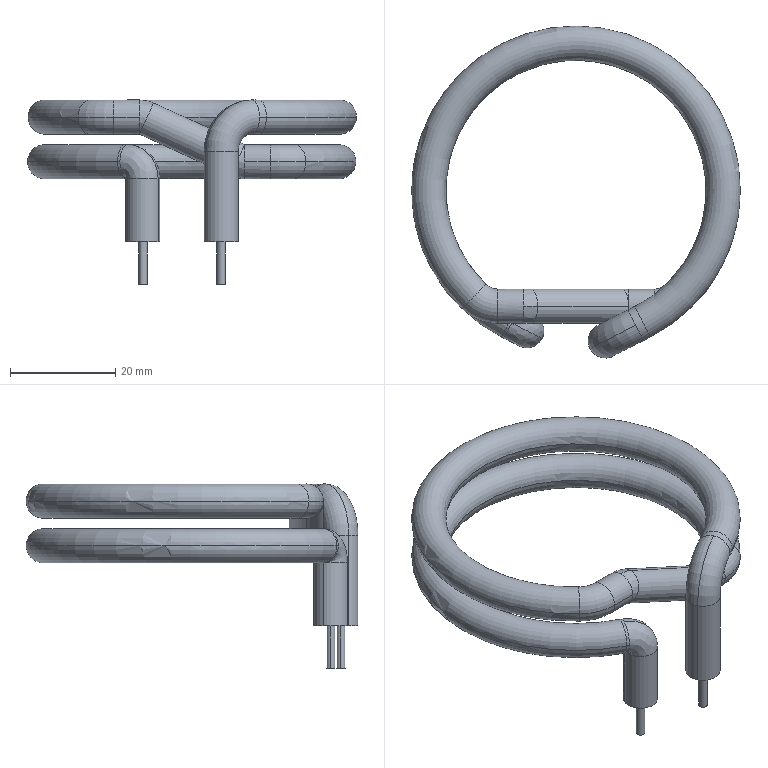Part | STEP file | JIAREQI_2_1_1_1 | 1 solid | 38 faces | box 62.5 x 63.088 x 35 mm | volume 12336 mm3 | cylinder 18 | torus 10 | spline 6 | plane 4 | commonest cylinder face diameters 6.5 x14 1.6 x4
STEP:
#1=CARTESIAN_POINT('',(0.,0.,0.));
#2=DIRECTION('',(0.,0.,1.));
#3=DIRECTION('',(1.,0.,0.));
#4=AXIS2_PLACEMENT_3D('',#1,#2,#3);
#5=CARTESIAN_POINT('',(11.339,-25.645,3.25));
#6=VERTEX_POINT('',#5);
#7=CARTESIAN_POINT('',(12.811,-28.543,0.));
#8=VERTEX_POINT('',#7);
#9=CARTESIAN_POINT('',(11.339,-25.645,0.));
#10=DIRECTION('',(0.8916,0.4527,0.));
#11=DIRECTION('',(0.,0.,1.));
#12=AXIS2_PLACEMENT_3D('',#9,#10,#11);
#13=CIRCLE('',#12,3.25);
#14=EDGE_CURVE('',#6,#8,#13,.T.);
#15=ORIENTED_EDGE('',*,*,#14,.F.);
#16=CARTESIAN_POINT('',(9.868,-22.747,0.));
#17=VERTEX_POINT('',#16);
#18=CARTESIAN_POINT('',(11.339,-25.645,0.));
#19=DIRECTION('',(0.8916,0.4527,0.));
#20=DIRECTION('',(-0.4527,0.8916,0.));
#21=AXIS2_PLACEMENT_3D('',#18,#19,#20);
#22=CIRCLE('',#21,3.25);
#23=EDGE_CURVE('',#17,#6,#22,.T.);
#24=ORIENTED_EDGE('',*,*,#23,.F.);
#25=CARTESIAN_POINT('',(11.206,-22.068,0.));
#26=VERTEX_POINT('',#25);
#27=CARTESIAN_POINT('',(9.868,-22.747,0.));
#28=DIRECTION('',(0.8916,0.4527,0.));
#29=VECTOR('',#28,1.5);
#30=LINE('',#27,#29);
#31=EDGE_CURVE('',#17,#26,#30,.T.);
#32=ORIENTED_EDGE('',*,*,#31,.T.);
#33=CARTESIAN_POINT('',(14.148,-27.864,0.));
#34=VERTEX_POINT('',#33);
#35=CARTESIAN_POINT('',(12.677,-24.966,0.));
#36=DIRECTION('',(-0.8916,-0.4527,0.));
#37=DIRECTION('',(0.4527,-0.8916,0.));
#38=AXIS2_PLACEMENT_3D('',#35,#36,#37);
#39=CIRCLE('',#38,3.25);
#40=EDGE_CURVE('',#34,#26,#39,.T.);
#41=ORIENTED_EDGE('',*,*,#40,.F.);
#42=CARTESIAN_POINT('',(12.811,-28.543,0.));
#43=DIRECTION('',(0.8916,0.4527,0.));
#44=VECTOR('',#43,1.5);
#45=LINE('',#42,#44);
#46=EDGE_CURVE('',#8,#34,#45,.T.);
#47=ORIENTED_EDGE('',*,*,#46,.F.);
#48=EDGE_LOOP('',(#15,#24,#32,#41,#47));
#49=FACE_OUTER_BOUND('',#48,.F.);
#50=CARTESIAN_POINT('',(11.339,-25.645,0.));
#51=DIRECTION('',(0.8916,0.4527,0.));
#52=DIRECTION('',(-0.4527,0.8916,0.));
#53=AXIS2_PLACEMENT_3D('',#50,#51,#52);
#54=CYLINDRICAL_SURFACE('',#53,3.25);
#55=ADVANCED_FACE('',(#49),#54,.T.);
#56=ORIENTED_EDGE('',*,*,#14,.T.);
#57=CARTESIAN_POINT('',(11.339,-25.645,-3.25));
#58=VERTEX_POINT('',#57);
#59=CARTESIAN_POINT('',(11.339,-25.645,0.));
#60=DIRECTION('',(0.8916,0.4527,0.));
#61=DIRECTION('',(0.4527,-0.8916,0.));
#62=AXIS2_PLACEMENT_3D('',#59,#60,#61);
#63=CIRCLE('',#62,3.25);
#64=EDGE_CURVE('',#8,#58,#63,.T.);
#65=ORIENTED_EDGE('',*,*,#64,.T.);
#66=CARTESIAN_POINT('',(8.442,-27.116,-6.5));
#67=VERTEX_POINT('',#66);
#68=CARTESIAN_POINT('',(11.339,-25.645,-6.5));
#69=DIRECTION('',(0.4527,-0.8916,0.));
#70=DIRECTION('',(0.,0.,1.));
#71=AXIS2_PLACEMENT_3D('',#68,#69,#70);
#72=CIRCLE('',#71,3.25);
#73=EDGE_CURVE('',#58,#67,#72,.T.);
#74=ORIENTED_EDGE('',*,*,#73,.T.);
#75=CARTESIAN_POINT('',(2.646,-30.059,-6.5));
#76=VERTEX_POINT('',#75);
#77=CARTESIAN_POINT('',(5.544,-28.588,-6.5));
#78=DIRECTION('',(0.,0.,-1.));
#79=DIRECTION('',(0.8916,0.4527,0.));
#80=AXIS2_PLACEMENT_3D('',#77,#78,#79);
#81=CIRCLE('',#80,3.25);
#82=EDGE_CURVE('',#67,#76,#81,.T.);
#83=ORIENTED_EDGE('',*,*,#82,.T.);
#84=CARTESIAN_POINT('',(11.339,-25.645,-6.5));
#85=DIRECTION('',(0.4527,-0.8916,0.));
#86=DIRECTION('',(0.,0.,1.));
#87=AXIS2_PLACEMENT_3D('',#84,#85,#86);
#88=CIRCLE('',#87,9.75);
#89=EDGE_CURVE('',#6,#76,#88,.T.);
#90=ORIENTED_EDGE('',*,*,#89,.F.);
#91=EDGE_LOOP('',(#56,#65,#74,#83,#90));
#92=FACE_OUTER_BOUND('',#91,.F.);
#93=CARTESIAN_POINT('',(11.339,-25.645,-6.5));
#94=DIRECTION('',(0.4527,-0.8916,0.));
#95=DIRECTION('',(0.,0.,-1.));
#96=AXIS2_PLACEMENT_3D('',#93,#94,#95);
#97=TOROIDAL_SURFACE('',#96,6.5,3.25);
#98=ADVANCED_FACE('',(#92),#97,.T.);
#99=ORIENTED_EDGE('',*,*,#64,.F.);
#100=ORIENTED_EDGE('',*,*,#46,.T.);
#101=CARTESIAN_POINT('',(12.677,-24.966,0.));
#102=DIRECTION('',(-0.8916,-0.4527,0.));
#103=DIRECTION('',(-0.4527,0.8916,0.));
#104=AXIS2_PLACEMENT_3D('',#101,#102,#103);
#105=CIRCLE('',#104,3.25);
#106=EDGE_CURVE('',#26,#34,#105,.T.);
#107=ORIENTED_EDGE('',*,*,#106,.F.);
#108=ORIENTED_EDGE('',*,*,#31,.F.);
#109=CARTESIAN_POINT('',(11.339,-25.645,0.));
#110=DIRECTION('',(0.8916,0.4527,0.));
#111=DIRECTION('',(0.,0.,-1.));
#112=AXIS2_PLACEMENT_3D('',#109,#110,#111);
#113=CIRCLE('',#112,3.25);
#114=EDGE_CURVE('',#58,#17,#113,.T.);
#115=ORIENTED_EDGE('',*,*,#114,.F.);
#116=EDGE_LOOP('',(#99,#100,#107,#108,#115));
#117=FACE_OUTER_BOUND('',#116,.F.);
#118=CARTESIAN_POINT('',(11.339,-25.645,0.));
#119=DIRECTION('',(0.8916,0.4527,0.));
#120=DIRECTION('',(-0.4527,0.8916,0.));
#121=AXIS2_PLACEMENT_3D('',#118,#119,#120);
#122=CYLINDRICAL_SURFACE('',#121,3.25);
#123=ADVANCED_FACE('',(#117),#122,.T.);
#124=ORIENTED_EDGE('',*,*,#106,.T.);
#125=CARTESIAN_POINT('',(-14.148,27.864,0.));
#126=VERTEX_POINT('',#125);
#127=CARTESIAN_POINT('',(0.,0.,0.));
#128=DIRECTION('',(0.,0.,1.));
#129=DIRECTION('',(0.4527,-0.8916,0.));
#130=AXIS2_PLACEMENT_3D('',#127,#128,#129);
#131=CIRCLE('',#130,31.25);
#132=EDGE_CURVE('',#34,#126,#131,.T.);
#133=ORIENTED_EDGE('',*,*,#132,.T.);
#134=CARTESIAN_POINT('',(-21.656,-22.529,0.));
#135=VERTEX_POINT('',#134);
#136=CARTESIAN_POINT('',(0.,0.,0.));
#137=DIRECTION('',(0.,0.,1.));
#138=DIRECTION('',(-0.4527,0.8916,0.));
#139=AXIS2_PLACEMENT_3D('',#136,#137,#138);
#140=CIRCLE('',#139,31.25);
#141=EDGE_CURVE('',#126,#135,#140,.T.);
#142=ORIENTED_EDGE('',*,*,#141,.T.);
#143=CARTESIAN_POINT('',(-17.152,-17.843,0.));
#144=VERTEX_POINT('',#143);
#145=CARTESIAN_POINT('',(-19.404,-20.186,0.));
#146=DIRECTION('',(0.7209,-0.693,0.));
#147=DIRECTION('',(-0.693,-0.7209,0.));
#148=AXIS2_PLACEMENT_3D('',#145,#146,#147);
#149=CIRCLE('',#148,3.25);
#150=EDGE_CURVE('',#135,#144,#149,.T.);
#151=ORIENTED_EDGE('',*,*,#150,.T.);
#152=CARTESIAN_POINT('',(-11.206,22.068,0.));
#153=VERTEX_POINT('',#152);
#154=CARTESIAN_POINT('',(0.,0.,0.));
#155=DIRECTION('',(0.,0.,1.));
#156=DIRECTION('',(-0.4527,0.8916,0.));
#157=AXIS2_PLACEMENT_3D('',#154,#155,#156);
#158=CIRCLE('',#157,24.75);
#159=EDGE_CURVE('',#153,#144,#158,.T.);
#160=ORIENTED_EDGE('',*,*,#159,.F.);
#161=CARTESIAN_POINT('',(0.,0.,0.));
#162=DIRECTION('',(0.,0.,1.));
#163=DIRECTION('',(0.4527,-0.8916,0.));
#164=AXIS2_PLACEMENT_3D('',#161,#162,#163);
#165=CIRCLE('',#164,24.75);
#166=EDGE_CURVE('',#26,#153,#165,.T.);
#167=ORIENTED_EDGE('',*,*,#166,.F.);
#168=EDGE_LOOP('',(#124,#133,#142,#151,#160,#167));
#169=FACE_OUTER_BOUND('',#168,.F.);
#170=CARTESIAN_POINT('',(0.,0.,0.));
#171=DIRECTION('',(0.,0.,1.));
#172=DIRECTION('',(-0.4527,0.8916,0.));
#173=AXIS2_PLACEMENT_3D('',#170,#171,#172);
#174=TOROIDAL_SURFACE('',#173,28.,3.25);
#175=ADVANCED_FACE('',(#169),#174,.T.);
#176=ORIENTED_EDGE('',*,*,#40,.T.);
#177=ORIENTED_EDGE('',*,*,#166,.T.);
#178=ORIENTED_EDGE('',*,*,#159,.T.);
#179=CARTESIAN_POINT('',(-19.404,-20.186,0.));
#180=DIRECTION('',(0.7209,-0.693,0.));
#181=DIRECTION('',(0.693,0.7209,0.));
#182=AXIS2_PLACEMENT_3D('',#179,#180,#181);
#183=CIRCLE('',#182,3.25);
#184=EDGE_CURVE('',#144,#135,#183,.T.);
#185=ORIENTED_EDGE('',*,*,#184,.T.);
#186=ORIENTED_EDGE('',*,*,#141,.F.);
#187=ORIENTED_EDGE('',*,*,#132,.F.);
#188=EDGE_LOOP('',(#176,#177,#178,#185,#186,#187));
#189=FACE_OUTER_BOUND('',#188,.F.);
#190=CARTESIAN_POINT('',(0.,0.,0.));
#191=DIRECTION('',(0.,0.,1.));
#192=DIRECTION('',(-0.4527,0.8916,0.));
#193=AXIS2_PLACEMENT_3D('',#190,#191,#192);
#194=TOROIDAL_SURFACE('',#193,28.,3.25);
#195=ADVANCED_FACE('',(#189),#194,.T.);
#196=ORIENTED_EDGE('',*,*,#184,.F.);
#197=CARTESIAN_POINT('',(-14.9,-18.75,0.));
#198=VERTEX_POINT('',#197);
#199=CARTESIAN_POINT('',(-14.9,-15.5,0.));
#200=DIRECTION('',(0.,0.,1.));
#201=DIRECTION('',(-0.693,-0.7209,0.));
#202=AXIS2_PLACEMENT_3D('',#199,#200,#201);
#203=CIRCLE('',#202,3.25);
#204=EDGE_CURVE('',#144,#198,#203,.T.);
#205=ORIENTED_EDGE('',*,*,#204,.T.);
#206=CARTESIAN_POINT('',(-14.9,-25.25,-0.00004664));
#207=VERTEX_POINT('',#206);
#208=CARTESIAN_POINT('',(-14.9,-22.,0.));
#209=DIRECTION('',(1.,0.,0.));
#210=DIRECTION('',(0.,1.,0.));
#211=AXIS2_PLACEMENT_3D('',#208,#209,#210);
#212=CIRCLE('',#211,3.25);
#213=EDGE_CURVE('',#198,#207,#212,.T.);
#214=ORIENTED_EDGE('',*,*,#213,.T.);
#215=CARTESIAN_POINT('',(-14.9,-15.5,0.));
#216=DIRECTION('',(0.,0.,1.));
#217=DIRECTION('',(-0.693,-0.7209,0.));
#218=AXIS2_PLACEMENT_3D('',#215,#216,#217);
#219=CIRCLE('',#218,9.75);
#220=EDGE_CURVE('',#135,#207,#219,.T.);
#221=ORIENTED_EDGE('',*,*,#220,.F.);
#222=EDGE_LOOP('',(#196,#205,#214,#221));
#223=FACE_OUTER_BOUND('',#222,.F.);
#224=CARTESIAN_POINT('',(-14.9,-15.5,0.));
#225=DIRECTION('',(0.,0.,1.));
#226=DIRECTION('',(0.693,0.7209,0.));
#227=AXIS2_PLACEMENT_3D('',#224,#225,#226);
#228=TOROIDAL_SURFACE('',#227,6.5,3.25);
#229=ADVANCED_FACE('',(#223),#228,.T.);
#230=ORIENTED_EDGE('',*,*,#150,.F.);
#231=ORIENTED_EDGE('',*,*,#220,.T.);
#232=CARTESIAN_POINT('',(-14.9,-22.,0.));
#233=DIRECTION('',(1.,0.,0.));
#234=DIRECTION('',(0.,-1.,-0.00001435));
#235=AXIS2_PLACEMENT_3D('',#232,#233,#234);
#236=CIRCLE('',#235,3.25);
#237=EDGE_CURVE('',#207,#198,#236,.T.);
#238=ORIENTED_EDGE('',*,*,#237,.T.);
#239=ORIENTED_EDGE('',*,*,#204,.F.);
#240=EDGE_LOOP('',(#230,#231,#238,#239));
#241=FACE_OUTER_BOUND('',#240,.F.);
#242=CARTESIAN_POINT('',(-14.9,-15.5,0.));
#243=DIRECTION('',(0.,0.,1.));
#244=DIRECTION('',(0.693,0.7209,0.));
#245=AXIS2_PLACEMENT_3D('',#242,#243,#244);
#246=TOROIDAL_SURFACE('',#245,6.5,3.25);
#247=ADVANCED_FACE('',(#241),#246,.T.);
#248=CARTESIAN_POINT('',(-10.,-18.75,-0.00003964));
#249=VERTEX_POINT('',#248);
#250=CARTESIAN_POINT('',(-14.9,-18.75,0.));
#251=DIRECTION('',(1.,0.,-0.000008091));
#252=VECTOR('',#251,4.9);
#253=LINE('',#250,#252);
#254=EDGE_CURVE('',#198,#249,#253,.T.);
#255=ORIENTED_EDGE('',*,*,#254,.F.);
#256=ORIENTED_EDGE('',*,*,#237,.F.);
#257=CARTESIAN_POINT('',(-10.,-25.25,-0.00008913));
#258=VERTEX_POINT('',#257);
#259=CARTESIAN_POINT('',(-14.9,-25.25,-0.00002332));
#260=DIRECTION('',(1.,0.,-0.00001343));
#261=VECTOR('',#260,4.9);
#262=LINE('',#259,#261);
#263=EDGE_CURVE('',#207,#258,#262,.T.);
#264=ORIENTED_EDGE('',*,*,#263,.T.);
#265=CARTESIAN_POINT('',(-10.,-22.,-3.25));
#266=VERTEX_POINT('',#265);
#267=CARTESIAN_POINT('',(-10.,-22.,0.));
#268=DIRECTION('',(-1.,0.,0.000001818));
#269=DIRECTION('',(-0.000001818,0.,-1.));
#270=AXIS2_PLACEMENT_3D('',#267,#268,#269);
#271=CIRCLE('',#270,3.25);
#272=EDGE_CURVE('',#266,#258,#271,.T.);
#273=ORIENTED_EDGE('',*,*,#272,.F.);
#274=CARTESIAN_POINT('',(-10.,-22.,0.));
#275=DIRECTION('',(-1.,0.,0.000001818));
#276=DIRECTION('',(0.,1.,0.));
#277=AXIS2_PLACEMENT_3D('',#274,#275,#276);
#278=CIRCLE('',#277,3.25);
#279=EDGE_CURVE('',#249,#266,#278,.T.);
#280=ORIENTED_EDGE('',*,*,#279,.F.);
#281=EDGE_LOOP('',(#255,#256,#264,#273,#280));
#282=FACE_OUTER_BOUND('',#281,.F.);
#283=CARTESIAN_POINT('',(-14.9,-22.,0.));
#284=DIRECTION('',(1.,0.,0.));
#285=DIRECTION('',(0.,1.,0.));
#286=AXIS2_PLACEMENT_3D('',#283,#284,#285);
#287=CYLINDRICAL_SURFACE('',#286,3.25);
#288=ADVANCED_FACE('',(#282),#287,.T.);
#289=ORIENTED_EDGE('',*,*,#254,.T.);
#290=CARTESIAN_POINT('',(-10.,-22.,3.25));
#291=VERTEX_POINT('',#290);
#292=CARTESIAN_POINT('',(-10.,-22.,0.));
#293=DIRECTION('',(-1.,0.,0.000001818));
#294=DIRECTION('',(0.000001818,0.,1.));
#295=AXIS2_PLACEMENT_3D('',#292,#293,#294);
#296=CIRCLE('',#295,3.25);
#297=EDGE_CURVE('',#291,#249,#296,.T.);
#298=ORIENTED_EDGE('',*,*,#297,.F.);
#299=CARTESIAN_POINT('',(-10.,-22.,0.));
#300=DIRECTION('',(-1.,0.,0.000001818));
#301=DIRECTION('',(0.,-1.,-0.00001435));
#302=AXIS2_PLACEMENT_3D('',#299,#300,#301);
#303=CIRCLE('',#302,3.25);
#304=EDGE_CURVE('',#258,#291,#303,.T.);
#305=ORIENTED_EDGE('',*,*,#304,.F.);
#306=ORIENTED_EDGE('',*,*,#263,.F.);
#307=ORIENTED_EDGE('',*,*,#213,.F.);
#308=EDGE_LOOP('',(#289,#298,#305,#306,#307));
#309=FACE_OUTER_BOUND('',#308,.F.);
#310=CARTESIAN_POINT('',(-14.9,-22.,0.));
#311=DIRECTION('',(1.,0.,0.));
#312=DIRECTION('',(0.,1.,0.));
#313=AXIS2_PLACEMENT_3D('',#310,#311,#312);
#314=CYLINDRICAL_SURFACE('',#313,3.25);
#315=ADVANCED_FACE('',(#309),#314,.T.);
#316=ORIENTED_EDGE('',*,*,#279,.T.);
#317=CARTESIAN_POINT('',(-7.296,-22.,2.661));
#318=VERTEX_POINT('',#317);
#319=CARTESIAN_POINT('',(-8.648,-22.,-0.2945));
#320=DIRECTION('',(0.9094,0.,-0.4159));
#321=DIRECTION('',(-0.4159,0.,-0.9094));
#322=AXIS2_PLACEMENT_3D('',#319,#320,#321);
#323=CIRCLE('',#322,3.25);
#324=EDGE_CURVE('',#266,#318,#323,.T.);
#325=ORIENTED_EDGE('',*,*,#324,.T.);
#326=CARTESIAN_POINT('',(-10.,-22.,-3.25));
#327=DIRECTION('',(0.,-1.,0.));
#328=DIRECTION('',(0.4159,0.,0.9094));
#329=AXIS2_PLACEMENT_3D('',#326,#327,#328);
#330=CIRCLE('',#329,6.5);
#331=EDGE_CURVE('',#318,#291,#330,.T.);
#332=ORIENTED_EDGE('',*,*,#331,.T.);
#333=ORIENTED_EDGE('',*,*,#297,.T.);
#334=EDGE_LOOP('',(#316,#325,#332,#333));
#335=FACE_OUTER_BOUND('',#334,.F.);
#336=CARTESIAN_POINT('',(-10.,-22.,-3.25));
#337=CARTESIAN_POINT('',(-10.,-20.048,-3.25));
#338=CARTESIAN_POINT('',(-9.395,-18.69,-1.986));
#339=CARTESIAN_POINT('',(-8.552,-18.752,-0.2269));
#340=CARTESIAN_POINT('',(-7.709,-18.813,1.532));
#341=CARTESIAN_POINT('',(-7.142,-20.256,2.717));
#342=CARTESIAN_POINT('',(-7.195,-22.204,2.606));
#343=CARTESIAN_POINT('',(-10.,-22.,-3.25));
#344=CARTESIAN_POINT('',(-10.,-20.048,-3.25));
#345=CARTESIAN_POINT('',(-9.592,-18.69,-1.891));
#346=CARTESIAN_POINT('',(-9.024,-18.752,-0.000618));
#347=CARTESIAN_POINT('',(-8.456,-18.813,1.89));
#348=CARTESIAN_POINT('',(-8.074,-20.256,3.163));
#349=CARTESIAN_POINT('',(-8.11,-22.204,3.045));
#350=CARTESIAN_POINT('',(-10.,-22.,-3.25));
#351=CARTESIAN_POINT('',(-10.,-20.048,-3.25));
#352=CARTESIAN_POINT('',(-9.806,-18.69,-1.845));
#353=CARTESIAN_POINT('',(-9.536,-18.752,0.1109));
#354=CARTESIAN_POINT('',(-9.266,-18.813,2.067));
#355=CARTESIAN_POINT('',(-9.084,-20.256,3.383));
#356=CARTESIAN_POINT('',(-9.101,-22.204,3.261));
#357=CARTESIAN_POINT('',(-10.,-22.,-3.25));
#358=CARTESIAN_POINT('',(-10.,-20.048,-3.25));
#359=CARTESIAN_POINT('',(-10.025,-18.69,-1.849));
#360=CARTESIAN_POINT('',(-10.06,-18.752,0.1016));
#361=CARTESIAN_POINT('',(-10.094,-18.813,2.052));
#362=CARTESIAN_POINT('',(-10.117,-20.256,3.365));
#363=CARTESIAN_POINT('',(-10.115,-22.204,3.243));
#364=(BOUNDED_SURFACE()B_SPLINE_SURFACE(3,3,((#336,#337,#338,#339,#340,#341,#342),(#343,#344,#345,#346,#347,#348,#349),(#350,#351,#352,#353,#354,#355,#356),(#357,#358,#359,#360,#361,#362,#363)),.UNSPECIFIED.,.F.,.F.,.F.)B_SPLINE_SURFACE_WITH_KNOTS((4,4),(4,3,4),(0.,1.),(0.,1.,2.),.UNSPECIFIED.)GEOMETRIC_REPRESENTATION_ITEM()RATIONAL_B_SPLINE_SURFACE(((1.195,0.953,0.953,1.195,0.953,0.953,1.195),(1.174,0.936,0.936,1.174,0.936,0.936,1.174),(1.174,0.936,0.936,1.174,0.936,0.936,1.174),(1.195,0.953,0.953,1.195,0.953,0.953,1.195)))REPRESENTATION_ITEM('')SURFACE());
#365=ADVANCED_FACE('',(#335),#364,.T.);
#366=CARTESIAN_POINT('',(10.,-22.,-5.25));
#367=VERTEX_POINT('',#366);
#368=CARTESIAN_POINT('',(7.296,-22.,-11.161));
#369=VERTEX_POINT('',#368);
#370=CARTESIAN_POINT('',(8.648,-22.,-8.206));
#371=DIRECTION('',(-0.9094,0.,0.4159));
#372=DIRECTION('',(0.4159,0.,0.9094));
#373=AXIS2_PLACEMENT_3D('',#370,#371,#372);
#374=CIRCLE('',#373,3.25);
#375=EDGE_CURVE('',#367,#369,#374,.T.);
#376=ORIENTED_EDGE('',*,*,#375,.F.);
#377=CARTESIAN_POINT('',(10.,-22.,-5.25));
#378=DIRECTION('',(-0.9094,0.,0.4159));
#379=VECTOR('',#378,19.02);
#380=LINE('',#377,#379);
#381=EDGE_CURVE('',#367,#318,#380,.T.);
#382=ORIENTED_EDGE('',*,*,#381,.T.);
#383=ORIENTED_EDGE('',*,*,#324,.F.);
#384=CARTESIAN_POINT('',(7.296,-22.,-11.161));
#385=DIRECTION('',(-0.9094,0.,0.4159));
#386=VECTOR('',#385,19.02);
#387=LINE('',#384,#386);
#388=EDGE_CURVE('',#369,#266,#387,.T.);
#389=ORIENTED_EDGE('',*,*,#388,.F.);
#390=EDGE_LOOP('',(#376,#382,#383,#389));
#391=FACE_OUTER_BOUND('',#390,.F.);
#392=CARTESIAN_POINT('',(8.648,-22.,-8.206));
#393=DIRECTION('',(-0.9094,0.,0.4159));
#394=DIRECTION('',(0.4159,0.,0.9094));
#395=AXIS2_PLACEMENT_3D('',#392,#393,#394);
#396=CYLINDRICAL_SURFACE('',#395,3.25);
#397=ADVANCED_FACE('',(#391),#396,.T.);
#398=CARTESIAN_POINT('',(10.,-22.,-11.75));
#399=VERTEX_POINT('',#398);
#400=CARTESIAN_POINT('',(10.,-18.75,-8.5));
#401=VERTEX_POINT('',#400);
#402=CARTESIAN_POINT('',(10.,-22.,-8.5));
#403=DIRECTION('',(1.,0.,-0.000001818));
#404=DIRECTION('',(-0.000001818,0.,-1.));
#405=AXIS2_PLACEMENT_3D('',#402,#403,#404);
#406=CIRCLE('',#405,3.25);
#407=EDGE_CURVE('',#399,#401,#406,.T.);
#408=ORIENTED_EDGE('',*,*,#407,.T.);
#409=CARTESIAN_POINT('',(10.,-22.,-8.5));
#410=DIRECTION('',(1.,0.,-0.000001818));
#411=DIRECTION('',(0.,1.,0.));
#412=AXIS2_PLACEMENT_3D('',#409,#410,#411);
#413=CIRCLE('',#412,3.25);
#414=EDGE_CURVE('',#401,#367,#413,.T.);
#415=ORIENTED_EDGE('',*,*,#414,.T.);
#416=ORIENTED_EDGE('',*,*,#375,.T.);
#417=CARTESIAN_POINT('',(10.,-22.,-5.25));
#418=DIRECTION('',(0.,1.,0.));
#419=DIRECTION('',(-0.000001818,0.,-1.));
#420=AXIS2_PLACEMENT_3D('',#417,#418,#419);
#421=CIRCLE('',#420,6.5);
#422=EDGE_CURVE('',#399,#369,#421,.T.);
#423=ORIENTED_EDGE('',*,*,#422,.F.);
#424=EDGE_LOOP('',(#408,#415,#416,#423));
#425=FACE_OUTER_BOUND('',#424,.F.);
#426=CARTESIAN_POINT('',(10.115,-22.204,-11.743));
#427=CARTESIAN_POINT('',(10.117,-20.256,-11.865));
#428=CARTESIAN_POINT('',(10.094,-18.813,-10.552));
#429=CARTESIAN_POINT('',(10.06,-18.752,-8.602));
#430=CARTESIAN_POINT('',(10.025,-18.69,-6.651));
#431=CARTESIAN_POINT('',(10.,-20.048,-5.25));
#432=CARTESIAN_POINT('',(10.,-22.,-5.25));
#433=CARTESIAN_POINT('',(9.101,-22.204,-11.761));
#434=CARTESIAN_POINT('',(9.084,-20.256,-11.883));
#435=CARTESIAN_POINT('',(9.266,-18.813,-10.567));
#436=CARTESIAN_POINT('',(9.536,-18.752,-8.611));
#437=CARTESIAN_POINT('',(9.806,-18.69,-6.655));
#438=CARTESIAN_POINT('',(10.,-20.048,-5.25));
#439=CARTESIAN_POINT('',(10.,-22.,-5.25));
#440=CARTESIAN_POINT('',(8.11,-22.204,-11.545));
#441=CARTESIAN_POINT('',(8.074,-20.256,-11.663));
#442=CARTESIAN_POINT('',(8.456,-18.813,-10.39));
#443=CARTESIAN_POINT('',(9.024,-18.752,-8.499));
#444=CARTESIAN_POINT('',(9.592,-18.69,-6.609));
#445=CARTESIAN_POINT('',(10.,-20.048,-5.25));
#446=CARTESIAN_POINT('',(10.,-22.,-5.25));
#447=CARTESIAN_POINT('',(7.195,-22.204,-11.106));
#448=CARTESIAN_POINT('',(7.142,-20.256,-11.217));
#449=CARTESIAN_POINT('',(7.709,-18.813,-10.032));
#450=CARTESIAN_POINT('',(8.552,-18.752,-8.273));
#451=CARTESIAN_POINT('',(9.395,-18.69,-6.514));
#452=CARTESIAN_POINT('',(10.,-20.048,-5.25));
#453=CARTESIAN_POINT('',(10.,-22.,-5.25));
#454=(BOUNDED_SURFACE()B_SPLINE_SURFACE(3,3,((#426,#427,#428,#429,#430,#431,#432),(#433,#434,#435,#436,#437,#438,#439),(#440,#441,#442,#443,#444,#445,#446),(#447,#448,#449,#450,#451,#452,#453)),.UNSPECIFIED.,.F.,.F.,.F.)B_SPLINE_SURFACE_WITH_KNOTS((4,4),(4,3,4),(0.,1.),(0.,1.,2.),.UNSPECIFIED.)GEOMETRIC_REPRESENTATION_ITEM()RATIONAL_B_SPLINE_SURFACE(((1.195,0.953,0.953,1.195,0.953,0.953,1.195),(1.174,0.936,0.936,1.174,0.936,0.936,1.174),(1.174,0.936,0.936,1.174,0.936,0.936,1.174),(1.195,0.953,0.953,1.195,0.953,0.953,1.195)))REPRESENTATION_ITEM('')SURFACE());
#455=ADVANCED_FACE('',(#425),#454,.T.);
#456=ORIENTED_EDGE('',*,*,#407,.F.);
#457=CARTESIAN_POINT('',(10.,-25.25,-8.5));
#458=VERTEX_POINT('',#457);
#459=CARTESIAN_POINT('',(10.,-22.,-8.5));
#460=DIRECTION('',(1.,0.,-0.000001818));
#461=DIRECTION('',(0.,-1.,0.00001275));
#462=AXIS2_PLACEMENT_3D('',#459,#460,#461);
#463=CIRCLE('',#462,3.25);
#464=EDGE_CURVE('',#458,#399,#463,.T.);
#465=ORIENTED_EDGE('',*,*,#464,.F.);
#466=CARTESIAN_POINT('',(14.9,-25.25,-8.5));
#467=VERTEX_POINT('',#466);
#468=CARTESIAN_POINT('',(14.9,-25.25,-8.5));
#469=DIRECTION('',(-1.,0.,0.00001163));
#470=VECTOR('',#469,4.9);
#471=LINE('',#468,#470);
#472=EDGE_CURVE('',#467,#458,#471,.T.);
#473=ORIENTED_EDGE('',*,*,#472,.F.);
#474=CARTESIAN_POINT('',(14.9,-18.75,-8.5));
#475=VERTEX_POINT('',#474);
#476=CARTESIAN_POINT('',(14.9,-22.,-8.5));
#477=DIRECTION('',(-1.,0.,0.));
#478=DIRECTION('',(0.,1.,0.));
#479=AXIS2_PLACEMENT_3D('',#476,#477,#478);
#480=CIRCLE('',#479,3.25);
#481=EDGE_CURVE('',#475,#467,#480,.T.);
#482=ORIENTED_EDGE('',*,*,#481,.F.);
#483=CARTESIAN_POINT('',(14.9,-18.75,-8.5));
#484=DIRECTION('',(-1.,0.,0.000008091));
#485=VECTOR('',#484,4.9);
#486=LINE('',#483,#485);
#487=EDGE_CURVE('',#475,#401,#486,.T.);
#488=ORIENTED_EDGE('',*,*,#487,.T.);
#489=EDGE_LOOP('',(#456,#465,#473,#482,#488));
#490=FACE_OUTER_BOUND('',#489,.F.);
#491=CARTESIAN_POINT('',(14.9,-22.,-8.5));
#492=DIRECTION('',(-1.,0.,0.));
#493=DIRECTION('',(0.,1.,0.));
#494=AXIS2_PLACEMENT_3D('',#491,#492,#493);
#495=CYLINDRICAL_SURFACE('',#494,3.25);
#496=ADVANCED_FACE('',(#490),#495,.T.);
#497=ORIENTED_EDGE('',*,*,#464,.T.);
#498=ORIENTED_EDGE('',*,*,#422,.T.);
#499=CARTESIAN_POINT('',(8.648,-22.,-8.206));
#500=DIRECTION('',(-0.9094,0.,0.4159));
#501=DIRECTION('',(-0.4159,0.,-0.9094));
#502=AXIS2_PLACEMENT_3D('',#499,#500,#501);
#503=CIRCLE('',#502,3.25);
#504=EDGE_CURVE('',#369,#367,#503,.T.);
#505=ORIENTED_EDGE('',*,*,#504,.T.);
#506=CARTESIAN_POINT('',(10.,-22.,-8.5));
#507=DIRECTION('',(1.,0.,-0.000001818));
#508=DIRECTION('',(0.000001818,0.,1.));
#509=AXIS2_PLACEMENT_3D('',#506,#507,#508);
#510=CIRCLE('',#509,3.25);
#511=EDGE_CURVE('',#367,#458,#510,.T.);
#512=ORIENTED_EDGE('',*,*,#511,.T.);
#513=EDGE_LOOP('',(#497,#498,#505,#512));
#514=FACE_OUTER_BOUND('',#513,.F.);
#515=CARTESIAN_POINT('',(10.,-22.,-5.25));
#516=CARTESIAN_POINT('',(10.,-23.952,-5.25));
#517=CARTESIAN_POINT('',(10.025,-25.31,-6.651));
#518=CARTESIAN_POINT('',(10.06,-25.248,-8.602));
#519=CARTESIAN_POINT('',(10.094,-25.187,-10.552));
#520=CARTESIAN_POINT('',(10.117,-23.744,-11.865));
#521=CARTESIAN_POINT('',(10.115,-21.796,-11.743));
#522=CARTESIAN_POINT('',(10.,-22.,-5.25));
#523=CARTESIAN_POINT('',(10.,-23.952,-5.25));
#524=CARTESIAN_POINT('',(9.806,-25.31,-6.655));
#525=CARTESIAN_POINT('',(9.536,-25.248,-8.611));
#526=CARTESIAN_POINT('',(9.266,-25.187,-10.567));
#527=CARTESIAN_POINT('',(9.084,-23.744,-11.883));
#528=CARTESIAN_POINT('',(9.101,-21.796,-11.761));
#529=CARTESIAN_POINT('',(10.,-22.,-5.25));
#530=CARTESIAN_POINT('',(10.,-23.952,-5.25));
#531=CARTESIAN_POINT('',(9.592,-25.31,-6.609));
#532=CARTESIAN_POINT('',(9.024,-25.248,-8.499));
#533=CARTESIAN_POINT('',(8.456,-25.187,-10.39));
#534=CARTESIAN_POINT('',(8.074,-23.744,-11.663));
#535=CARTESIAN_POINT('',(8.11,-21.796,-11.545));
#536=CARTESIAN_POINT('',(10.,-22.,-5.25));
#537=CARTESIAN_POINT('',(10.,-23.952,-5.25));
#538=CARTESIAN_POINT('',(9.395,-25.31,-6.514));
#539=CARTESIAN_POINT('',(8.552,-25.248,-8.273));
#540=CARTESIAN_POINT('',(7.709,-25.187,-10.032));
#541=CARTESIAN_POINT('',(7.142,-23.744,-11.217));
#542=CARTESIAN_POINT('',(7.195,-21.796,-11.106));
#543=(BOUNDED_SURFACE()B_SPLINE_SURFACE(3,3,((#515,#516,#517,#518,#519,#520,#521),(#522,#523,#524,#525,#526,#527,#528),(#529,#530,#531,#532,#533,#534,#535),(#536,#537,#538,#539,#540,#541,#542)),.UNSPECIFIED.,.F.,.F.,.F.)B_SPLINE_SURFACE_WITH_KNOTS((4,4),(4,3,4),(0.,1.),(0.,1.,2.),.UNSPECIFIED.)GEOMETRIC_REPRESENTATION_ITEM()RATIONAL_B_SPLINE_SURFACE(((1.195,0.953,0.953,1.195,0.953,0.953,1.195),(1.174,0.936,0.936,1.174,0.936,0.936,1.174),(1.174,0.936,0.936,1.174,0.936,0.936,1.174),(1.195,0.953,0.953,1.195,0.953,0.953,1.195)))REPRESENTATION_ITEM('')SURFACE());
#544=ADVANCED_FACE('',(#514),#543,.T.);
#545=ORIENTED_EDGE('',*,*,#504,.F.);
#546=ORIENTED_EDGE('',*,*,#388,.T.);
#547=CARTESIAN_POINT('',(-8.648,-22.,-0.2945));
#548=DIRECTION('',(0.9094,0.,-0.4159));
#549=DIRECTION('',(0.4159,0.,0.9094));
#550=AXIS2_PLACEMENT_3D('',#547,#548,#549);
#551=CIRCLE('',#550,3.25);
#552=EDGE_CURVE('',#318,#266,#551,.T.);
#553=ORIENTED_EDGE('',*,*,#552,.F.);
#554=ORIENTED_EDGE('',*,*,#381,.F.);
#555=EDGE_LOOP('',(#545,#546,#553,#554));
#556=FACE_OUTER_BOUND('',#555,.F.);
#557=CARTESIAN_POINT('',(8.648,-22.,-8.206));
#558=DIRECTION('',(-0.9094,0.,0.4159));
#559=DIRECTION('',(0.4159,0.,0.9094));
#560=AXIS2_PLACEMENT_3D('',#557,#558,#559);
#561=CYLINDRICAL_SURFACE('',#560,3.25);
#562=ADVANCED_FACE('',(#556),#561,.T.);
#563=ORIENTED_EDGE('',*,*,#304,.T.);
#564=ORIENTED_EDGE('',*,*,#331,.F.);
#565=ORIENTED_EDGE('',*,*,#552,.T.);
#566=ORIENTED_EDGE('',*,*,#272,.T.);
#567=EDGE_LOOP('',(#563,#564,#565,#566));
#568=FACE_OUTER_BOUND('',#567,.F.);
#569=CARTESIAN_POINT('',(-7.195,-21.796,2.606));
#570=CARTESIAN_POINT('',(-7.142,-23.744,2.717));
#571=CARTESIAN_POINT('',(-7.709,-25.187,1.532));
#572=CARTESIAN_POINT('',(-8.552,-25.248,-0.2269));
#573=CARTESIAN_POINT('',(-9.395,-25.31,-1.986));
#574=CARTESIAN_POINT('',(-10.,-23.952,-3.25));
#575=CARTESIAN_POINT('',(-10.,-22.,-3.25));
#576=CARTESIAN_POINT('',(-8.11,-21.796,3.045));
#577=CARTESIAN_POINT('',(-8.074,-23.744,3.163));
#578=CARTESIAN_POINT('',(-8.456,-25.187,1.89));
#579=CARTESIAN_POINT('',(-9.024,-25.248,-0.000618));
#580=CARTESIAN_POINT('',(-9.592,-25.31,-1.891));
#581=CARTESIAN_POINT('',(-10.,-23.952,-3.25));
#582=CARTESIAN_POINT('',(-10.,-22.,-3.25));
#583=CARTESIAN_POINT('',(-9.101,-21.796,3.261));
#584=CARTESIAN_POINT('',(-9.084,-23.744,3.383));
#585=CARTESIAN_POINT('',(-9.266,-25.187,2.067));
#586=CARTESIAN_POINT('',(-9.536,-25.248,0.1109));
#587=CARTESIAN_POINT('',(-9.806,-25.31,-1.845));
#588=CARTESIAN_POINT('',(-10.,-23.952,-3.25));
#589=CARTESIAN_POINT('',(-10.,-22.,-3.25));
#590=CARTESIAN_POINT('',(-10.115,-21.796,3.243));
#591=CARTESIAN_POINT('',(-10.117,-23.744,3.365));
#592=CARTESIAN_POINT('',(-10.094,-25.187,2.052));
#593=CARTESIAN_POINT('',(-10.06,-25.248,0.1016));
#594=CARTESIAN_POINT('',(-10.025,-25.31,-1.849));
#595=CARTESIAN_POINT('',(-10.,-23.952,-3.25));
#596=CARTESIAN_POINT('',(-10.,-22.,-3.25));
#597=(BOUNDED_SURFACE()B_SPLINE_SURFACE(3,3,((#569,#570,#571,#572,#573,#574,#575),(#576,#577,#578,#579,#580,#581,#582),(#583,#584,#585,#586,#587,#588,#589),(#590,#591,#592,#593,#594,#595,#596)),.UNSPECIFIED.,.F.,.F.,.F.)B_SPLINE_SURFACE_WITH_KNOTS((4,4),(4,3,4),(0.,1.),(0.,1.,2.),.UNSPECIFIED.)GEOMETRIC_REPRESENTATION_ITEM()RATIONAL_B_SPLINE_SURFACE(((1.195,0.953,0.953,1.195,0.953,0.953,1.195),(1.174,0.936,0.936,1.174,0.936,0.936,1.174),(1.174,0.936,0.936,1.174,0.936,0.936,1.174),(1.195,0.953,0.953,1.195,0.953,0.953,1.195)))REPRESENTATION_ITEM('')SURFACE());
#598=ADVANCED_FACE('',(#568),#597,.T.);
#599=ORIENTED_EDGE('',*,*,#511,.F.);
#600=ORIENTED_EDGE('',*,*,#414,.F.);
#601=ORIENTED_EDGE('',*,*,#487,.F.);
#602=CARTESIAN_POINT('',(14.9,-22.,-8.5));
#603=DIRECTION('',(-1.,0.,0.));
#604=DIRECTION('',(0.,-1.,0.00001275));
#605=AXIS2_PLACEMENT_3D('',#602,#603,#604);
#606=CIRCLE('',#605,3.25);
#607=EDGE_CURVE('',#467,#475,#606,.T.);
#608=ORIENTED_EDGE('',*,*,#607,.F.);
#609=ORIENTED_EDGE('',*,*,#472,.T.);
#610=EDGE_LOOP('',(#599,#600,#601,#608,#609));
#611=FACE_OUTER_BOUND('',#610,.F.);
#612=CARTESIAN_POINT('',(14.9,-22.,-8.5));
#613=DIRECTION('',(-1.,0.,0.));
#614=DIRECTION('',(0.,1.,0.));
#615=AXIS2_PLACEMENT_3D('',#612,#613,#614);
#616=CYLINDRICAL_SURFACE('',#615,3.25);
#617=ADVANCED_FACE('',(#611),#616,.T.);
#618=CARTESIAN_POINT('',(21.656,-22.529,-8.5));
#619=VERTEX_POINT('',#618);
#620=CARTESIAN_POINT('',(17.152,-17.843,-8.5));
#621=VERTEX_POINT('',#620);
#622=CARTESIAN_POINT('',(19.404,-20.186,-8.5));
#623=DIRECTION('',(-0.7209,-0.693,0.));
#624=DIRECTION('',(0.693,-0.7209,0.));
#625=AXIS2_PLACEMENT_3D('',#622,#623,#624);
#626=CIRCLE('',#625,3.25);
#627=EDGE_CURVE('',#619,#621,#626,.T.);
#628=ORIENTED_EDGE('',*,*,#627,.F.);
#629=CARTESIAN_POINT('',(14.9,-15.5,-8.5));
#630=DIRECTION('',(0.,0.,-1.));
#631=DIRECTION('',(0.693,-0.7209,0.));
#632=AXIS2_PLACEMENT_3D('',#629,#630,#631);
#633=CIRCLE('',#632,9.75);
#634=EDGE_CURVE('',#619,#467,#633,.T.);
#635=ORIENTED_EDGE('',*,*,#634,.T.);
#636=ORIENTED_EDGE('',*,*,#607,.T.);
#637=CARTESIAN_POINT('',(14.9,-15.5,-8.5));
#638=DIRECTION('',(0.,0.,-1.));
#639=DIRECTION('',(0.693,-0.7209,0.));
#640=AXIS2_PLACEMENT_3D('',#637,#638,#639);
#641=CIRCLE('',#640,3.25);
#642=EDGE_CURVE('',#621,#475,#641,.T.);
#643=ORIENTED_EDGE('',*,*,#642,.F.);
#644=EDGE_LOOP('',(#628,#635,#636,#643));
#645=FACE_OUTER_BOUND('',#644,.F.);
#646=CARTESIAN_POINT('',(14.9,-15.5,-8.5));
#647=DIRECTION('',(0.,0.,-1.));
#648=DIRECTION('',(-0.693,0.7209,0.));
#649=AXIS2_PLACEMENT_3D('',#646,#647,#648);
#650=TOROIDAL_SURFACE('',#649,6.5,3.25);
#651=ADVANCED_FACE('',(#645),#650,.T.);
#652=CARTESIAN_POINT('',(-14.148,-27.864,-8.5));
#653=VERTEX_POINT('',#652);
#654=CARTESIAN_POINT('',(14.148,27.864,-8.5));
#655=VERTEX_POINT('',#654);
#656=CARTESIAN_POINT('',(0.,0.,-8.5));
#657=DIRECTION('',(0.,0.,-1.));
#658=DIRECTION('',(-0.4527,-0.8916,0.));
#659=AXIS2_PLACEMENT_3D('',#656,#657,#658);
#660=CIRCLE('',#659,31.25);
#661=EDGE_CURVE('',#653,#655,#660,.T.);
#662=ORIENTED_EDGE('',*,*,#661,.T.);
#663=CARTESIAN_POINT('',(0.,0.,-8.5));
#664=DIRECTION('',(0.,0.,-1.));
#665=DIRECTION('',(0.4527,0.8916,0.));
#666=AXIS2_PLACEMENT_3D('',#663,#664,#665);
#667=CIRCLE('',#666,31.25);
#668=EDGE_CURVE('',#655,#619,#667,.T.);
#669=ORIENTED_EDGE('',*,*,#668,.T.);
#670=ORIENTED_EDGE('',*,*,#627,.T.);
#671=CARTESIAN_POINT('',(11.206,22.068,-8.5));
#672=VERTEX_POINT('',#671);
#673=CARTESIAN_POINT('',(0.,0.,-8.5));
#674=DIRECTION('',(0.,0.,1.));
#675=DIRECTION('',(0.693,-0.7209,0.));
#676=AXIS2_PLACEMENT_3D('',#673,#674,#675);
#677=CIRCLE('',#676,24.75);
#678=EDGE_CURVE('',#621,#672,#677,.T.);
#679=ORIENTED_EDGE('',*,*,#678,.T.);
#680=CARTESIAN_POINT('',(-11.206,-22.068,-8.5));
#681=VERTEX_POINT('',#680);
#682=CARTESIAN_POINT('',(0.,0.,-8.5));
#683=DIRECTION('',(0.,0.,1.));
#684=DIRECTION('',(0.4527,0.8916,0.));
#685=AXIS2_PLACEMENT_3D('',#682,#683,#684);
#686=CIRCLE('',#685,24.75);
#687=EDGE_CURVE('',#672,#681,#686,.T.);
#688=ORIENTED_EDGE('',*,*,#687,.T.);
#689=CARTESIAN_POINT('',(-12.677,-24.966,-8.5));
#690=DIRECTION('',(0.8916,-0.4527,0.));
#691=DIRECTION('',(0.4527,0.8916,0.));
#692=AXIS2_PLACEMENT_3D('',#689,#690,#691);
#693=CIRCLE('',#692,3.25);
#694=EDGE_CURVE('',#681,#653,#693,.T.);
#695=ORIENTED_EDGE('',*,*,#694,.T.);
#696=EDGE_LOOP('',(#662,#669,#670,#679,#688,#695));
#697=FACE_OUTER_BOUND('',#696,.F.);
#698=CARTESIAN_POINT('',(0.,0.,-8.5));
#699=DIRECTION('',(0.,0.,-1.));
#700=DIRECTION('',(0.4527,0.8916,0.));
#701=AXIS2_PLACEMENT_3D('',#698,#699,#700);
#702=TOROIDAL_SURFACE('',#701,28.,3.25);
#703=ADVANCED_FACE('',(#697),#702,.T.);
#704=ORIENTED_EDGE('',*,*,#687,.F.);
#705=ORIENTED_EDGE('',*,*,#678,.F.);
#706=CARTESIAN_POINT('',(19.404,-20.186,-8.5));
#707=DIRECTION('',(-0.7209,-0.693,0.));
#708=DIRECTION('',(-0.693,0.7209,0.));
#709=AXIS2_PLACEMENT_3D('',#706,#707,#708);
#710=CIRCLE('',#709,3.25);
#711=EDGE_CURVE('',#621,#619,#710,.T.);
#712=ORIENTED_EDGE('',*,*,#711,.T.);
#713=ORIENTED_EDGE('',*,*,#668,.F.);
#714=ORIENTED_EDGE('',*,*,#661,.F.);
#715=CARTESIAN_POINT('',(-12.677,-24.966,-8.5));
#716=DIRECTION('',(0.8916,-0.4527,0.));
#717=DIRECTION('',(-0.4527,-0.8916,-0.00007615));
#718=AXIS2_PLACEMENT_3D('',#715,#716,#717);
#719=CIRCLE('',#718,3.25);
#720=EDGE_CURVE('',#653,#681,#719,.T.);
#721=ORIENTED_EDGE('',*,*,#720,.T.);
#722=EDGE_LOOP('',(#704,#705,#712,#713,#714,#721));
#723=FACE_OUTER_BOUND('',#722,.F.);
#724=CARTESIAN_POINT('',(0.,0.,-8.5));
#725=DIRECTION('',(0.,0.,-1.));
#726=DIRECTION('',(0.4527,0.8916,0.));
#727=AXIS2_PLACEMENT_3D('',#724,#725,#726);
#728=TOROIDAL_SURFACE('',#727,28.,3.25);
#729=ADVANCED_FACE('',(#723),#728,.T.);
#730=ORIENTED_EDGE('',*,*,#711,.F.);
#731=ORIENTED_EDGE('',*,*,#642,.T.);
#732=ORIENTED_EDGE('',*,*,#481,.T.);
#733=ORIENTED_EDGE('',*,*,#634,.F.);
#734=EDGE_LOOP('',(#730,#731,#732,#733));
#735=FACE_OUTER_BOUND('',#734,.F.);
#736=CARTESIAN_POINT('',(14.9,-15.5,-8.5));
#737=DIRECTION('',(0.,0.,-1.));
#738=DIRECTION('',(-0.693,0.7209,0.));
#739=AXIS2_PLACEMENT_3D('',#736,#737,#738);
#740=TOROIDAL_SURFACE('',#739,6.5,3.25);
#741=ADVANCED_FACE('',(#735),#740,.T.);
#742=CARTESIAN_POINT('',(-10.76,-22.294,-8.5));
#743=VERTEX_POINT('',#742);
#744=CARTESIAN_POINT('',(-12.231,-25.192,-11.75));
#745=VERTEX_POINT('',#744);
#746=CARTESIAN_POINT('',(-12.231,-25.192,-8.5));
#747=DIRECTION('',(-0.8916,0.4527,0.00001408));
#748=DIRECTION('',(0.4527,0.8916,0.));
#749=AXIS2_PLACEMENT_3D('',#746,#747,#748);
#750=CIRCLE('',#749,3.25);
#751=EDGE_CURVE('',#743,#745,#750,.T.);
#752=ORIENTED_EDGE('',*,*,#751,.F.);
#753=CARTESIAN_POINT('',(-10.76,-22.294,-8.5));
#754=DIRECTION('',(-0.8916,0.4527,0.0003702));
#755=VECTOR('',#754,0.5);
#756=LINE('',#753,#755);
#757=EDGE_CURVE('',#743,#681,#756,.T.);
#758=ORIENTED_EDGE('',*,*,#757,.T.);
#759=ORIENTED_EDGE('',*,*,#720,.F.);
#760=CARTESIAN_POINT('',(-13.703,-28.09,-8.5));
#761=VERTEX_POINT('',#760);
#762=CARTESIAN_POINT('',(-13.703,-28.09,-8.5));
#763=DIRECTION('',(-0.8916,0.4527,0.0007237));
#764=VECTOR('',#763,0.5);
#765=LINE('',#762,#764);
#766=EDGE_CURVE('',#761,#653,#765,.T.);
#767=ORIENTED_EDGE('',*,*,#766,.F.);
#768=CARTESIAN_POINT('',(-12.231,-25.192,-8.5));
#769=DIRECTION('',(-0.8916,0.4527,0.00001408));
#770=DIRECTION('',(-0.00001256,0.000006376,-1.));
#771=AXIS2_PLACEMENT_3D('',#768,#769,#770);
#772=CIRCLE('',#771,3.25);
#773=EDGE_CURVE('',#745,#761,#772,.T.);
#774=ORIENTED_EDGE('',*,*,#773,.F.);
#775=EDGE_LOOP('',(#752,#758,#759,#767,#774));
#776=FACE_OUTER_BOUND('',#775,.F.);
#777=CARTESIAN_POINT('',(-12.231,-25.192,-8.5));
#778=DIRECTION('',(-0.8916,0.4527,0.));
#779=DIRECTION('',(0.4527,0.8916,0.));
#780=AXIS2_PLACEMENT_3D('',#777,#778,#779);
#781=CYLINDRICAL_SURFACE('',#780,3.25);
#782=ADVANCED_FACE('',(#776),#781,.T.);
#783=CARTESIAN_POINT('',(-12.231,-25.192,-5.25));
#784=VERTEX_POINT('',#783);
#785=CARTESIAN_POINT('',(-12.231,-25.192,-8.5));
#786=DIRECTION('',(-0.8916,0.4527,0.00001408));
#787=DIRECTION('',(0.00001256,-0.000006376,1.));
#788=AXIS2_PLACEMENT_3D('',#785,#786,#787);
#789=CIRCLE('',#788,3.25);
#790=EDGE_CURVE('',#784,#743,#789,.T.);
#791=ORIENTED_EDGE('',*,*,#790,.T.);
#792=ORIENTED_EDGE('',*,*,#751,.T.);
#793=CARTESIAN_POINT('',(-6.435,-28.135,-11.75));
#794=VERTEX_POINT('',#793);
#795=CARTESIAN_POINT('',(-9.333,-26.664,-11.75));
#796=DIRECTION('',(0.,0.,-1.));
#797=DIRECTION('',(-0.8916,0.4527,0.));
#798=AXIS2_PLACEMENT_3D('',#795,#796,#797);
#799=CIRCLE('',#798,3.25);
#800=EDGE_CURVE('',#745,#794,#799,.T.);
#801=ORIENTED_EDGE('',*,*,#800,.T.);
#802=CARTESIAN_POINT('',(-12.231,-25.192,-11.75));
#803=DIRECTION('',(0.4527,0.8916,0.));
#804=DIRECTION('',(0.00001256,-0.000006376,1.));
#805=AXIS2_PLACEMENT_3D('',#802,#803,#804);
#806=CIRCLE('',#805,6.5);
#807=EDGE_CURVE('',#784,#794,#806,.T.);
#808=ORIENTED_EDGE('',*,*,#807,.F.);
#809=EDGE_LOOP('',(#791,#792,#801,#808));
#810=FACE_OUTER_BOUND('',#809,.F.);
#811=CARTESIAN_POINT('',(-12.505,-25.282,-5.26));
#812=CARTESIAN_POINT('',(-11.627,-23.543,-5.137));
#813=CARTESIAN_POINT('',(-10.937,-22.275,-6.45));
#814=CARTESIAN_POINT('',(-10.854,-22.248,-8.4));
#815=CARTESIAN_POINT('',(-10.772,-22.221,-10.349));
#816=CARTESIAN_POINT('',(-11.348,-23.452,-11.75));
#817=CARTESIAN_POINT('',(-12.231,-25.192,-11.75));
#818=CARTESIAN_POINT('',(-8.944,-27.09,-5.134));
#819=CARTESIAN_POINT('',(-7.998,-25.386,-5.009));
#820=CARTESIAN_POINT('',(-8.028,-23.752,-6.347));
#821=CARTESIAN_POINT('',(-9.016,-23.182,-8.335));
#822=CARTESIAN_POINT('',(-10.003,-22.612,-10.322));
#823=CARTESIAN_POINT('',(-11.348,-23.452,-11.75));
#824=CARTESIAN_POINT('',(-12.231,-25.192,-11.75));
#825=CARTESIAN_POINT('',(-6.425,-28.37,-7.96));
#826=CARTESIAN_POINT('',(-5.431,-26.689,-7.888));
#827=CARTESIAN_POINT('',(-5.971,-24.797,-8.655));
#828=CARTESIAN_POINT('',(-7.715,-23.842,-9.793));
#829=CARTESIAN_POINT('',(-9.46,-22.888,-10.932));
#830=CARTESIAN_POINT('',(-11.348,-23.452,-11.75));
#831=CARTESIAN_POINT('',(-12.231,-25.192,-11.75));
#832=CARTESIAN_POINT('',(-6.536,-28.313,-11.954));
#833=CARTESIAN_POINT('',(-5.545,-26.632,-11.958));
#834=CARTESIAN_POINT('',(-6.062,-24.75,-11.917));
#835=CARTESIAN_POINT('',(-7.773,-23.813,-11.855));
#836=CARTESIAN_POINT('',(-9.484,-22.875,-11.794));
#837=CARTESIAN_POINT('',(-11.348,-23.452,-11.75));
#838=CARTESIAN_POINT('',(-12.231,-25.192,-11.75));
#839=(BOUNDED_SURFACE()B_SPLINE_SURFACE(3,3,((#811,#812,#813,#814,#815,#816,#817),(#818,#819,#820,#821,#822,#823,#824),(#825,#826,#827,#828,#829,#830,#831),(#832,#833,#834,#835,#836,#837,#838)),.UNSPECIFIED.,.F.,.F.,.F.)B_SPLINE_SURFACE_WITH_KNOTS((4,4),(4,3,4),(0.,1.),(0.,1.,2.),.UNSPECIFIED.)GEOMETRIC_REPRESENTATION_ITEM()RATIONAL_B_SPLINE_SURFACE(((1.4,1.116,1.116,1.4,1.116,1.116,1.4),(1.106,0.8815,0.8815,1.106,0.8815,0.8815,1.106),(1.106,0.8815,0.8815,1.106,0.8815,0.8815,1.106),(1.4,1.116,1.116,1.4,1.116,1.116,1.4)))REPRESENTATION_ITEM('')SURFACE());
#840=ADVANCED_FACE('',(#810),#839,.T.);
#841=ORIENTED_EDGE('',*,*,#790,.F.);
#842=CARTESIAN_POINT('',(-12.231,-25.192,-8.5));
#843=DIRECTION('',(-0.8916,0.4527,0.00001408));
#844=DIRECTION('',(-0.4527,-0.8916,-0.00007615));
#845=AXIS2_PLACEMENT_3D('',#842,#843,#844);
#846=CIRCLE('',#845,3.25);
#847=EDGE_CURVE('',#761,#784,#846,.T.);
#848=ORIENTED_EDGE('',*,*,#847,.F.);
#849=ORIENTED_EDGE('',*,*,#766,.T.);
#850=ORIENTED_EDGE('',*,*,#694,.F.);
#851=ORIENTED_EDGE('',*,*,#757,.F.);
#852=EDGE_LOOP('',(#841,#848,#849,#850,#851));
#853=FACE_OUTER_BOUND('',#852,.F.);
#854=CARTESIAN_POINT('',(-12.231,-25.192,-8.5));
#855=DIRECTION('',(-0.8916,0.4527,0.));
#856=DIRECTION('',(0.4527,0.8916,0.));
#857=AXIS2_PLACEMENT_3D('',#854,#855,#856);
#858=CYLINDRICAL_SURFACE('',#857,3.25);
#859=ADVANCED_FACE('',(#853),#858,.T.);
#860=ORIENTED_EDGE('',*,*,#773,.T.);
#861=ORIENTED_EDGE('',*,*,#847,.T.);
#862=ORIENTED_EDGE('',*,*,#807,.T.);
#863=CARTESIAN_POINT('',(-9.333,-26.664,-11.75));
#864=DIRECTION('',(0.,0.,-1.));
#865=DIRECTION('',(0.8916,-0.4527,0.));
#866=AXIS2_PLACEMENT_3D('',#863,#864,#865);
#867=CIRCLE('',#866,3.25);
#868=EDGE_CURVE('',#794,#745,#867,.T.);
#869=ORIENTED_EDGE('',*,*,#868,.T.);
#870=EDGE_LOOP('',(#860,#861,#862,#869));
#871=FACE_OUTER_BOUND('',#870,.F.);
#872=CARTESIAN_POINT('',(-12.231,-25.192,-11.75));
#873=CARTESIAN_POINT('',(-13.115,-26.932,-11.75));
#874=CARTESIAN_POINT('',(-13.769,-28.123,-10.349));
#875=CARTESIAN_POINT('',(-13.796,-28.041,-8.4));
#876=CARTESIAN_POINT('',(-13.823,-27.959,-6.45));
#877=CARTESIAN_POINT('',(-13.206,-26.653,-5.137));
#878=CARTESIAN_POINT('',(-12.321,-24.918,-5.26));
#879=CARTESIAN_POINT('',(-12.231,-25.192,-11.75));
#880=CARTESIAN_POINT('',(-13.115,-26.932,-11.75));
#881=CARTESIAN_POINT('',(-13.,-28.514,-10.322));
#882=CARTESIAN_POINT('',(-11.957,-28.974,-8.335));
#883=CARTESIAN_POINT('',(-10.914,-29.435,-6.347));
#884=CARTESIAN_POINT('',(-9.577,-28.495,-5.009));
#885=CARTESIAN_POINT('',(-8.759,-26.726,-5.134));
#886=CARTESIAN_POINT('',(-12.231,-25.192,-11.75));
#887=CARTESIAN_POINT('',(-13.115,-26.932,-11.75));
#888=CARTESIAN_POINT('',(-12.456,-28.79,-10.932));
#889=CARTESIAN_POINT('',(-10.657,-29.635,-9.793));
#890=CARTESIAN_POINT('',(-8.857,-30.48,-8.655));
#891=CARTESIAN_POINT('',(-7.01,-29.799,-7.888));
#892=CARTESIAN_POINT('',(-6.24,-28.006,-7.96));
#893=CARTESIAN_POINT('',(-12.231,-25.192,-11.75));
#894=CARTESIAN_POINT('',(-13.115,-26.932,-11.75));
#895=CARTESIAN_POINT('',(-12.481,-28.778,-11.794));
#896=CARTESIAN_POINT('',(-10.714,-29.606,-11.855));
#897=CARTESIAN_POINT('',(-8.948,-30.434,-11.917));
#898=CARTESIAN_POINT('',(-7.124,-29.741,-11.958));
#899=CARTESIAN_POINT('',(-6.352,-27.949,-11.954));
#900=(BOUNDED_SURFACE()B_SPLINE_SURFACE(3,3,((#872,#873,#874,#875,#876,#877,#878),(#879,#880,#881,#882,#883,#884,#885),(#886,#887,#888,#889,#890,#891,#892),(#893,#894,#895,#896,#897,#898,#899)),.UNSPECIFIED.,.F.,.F.,.F.)B_SPLINE_SURFACE_WITH_KNOTS((4,4),(4,3,4),(0.,1.),(0.,1.,2.),.UNSPECIFIED.)GEOMETRIC_REPRESENTATION_ITEM()RATIONAL_B_SPLINE_SURFACE(((1.4,1.116,1.116,1.4,1.116,1.116,1.4),(1.106,0.8815,0.8815,1.106,0.8815,0.8815,1.106),(1.106,0.8815,0.8815,1.106,0.8815,0.8815,1.106),(1.4,1.116,1.116,1.4,1.116,1.116,1.4)))REPRESENTATION_ITEM('')SURFACE());
#901=ADVANCED_FACE('',(#871),#900,.T.);
#902=ORIENTED_EDGE('',*,*,#868,.F.);
#903=CARTESIAN_POINT('',(-6.435,-28.135,-23.75));
#904=VERTEX_POINT('',#903);
#905=CARTESIAN_POINT('',(-6.435,-28.135,-11.75));
#906=DIRECTION('',(0.,0.,-1.));
#907=VECTOR('',#906,12.);
#908=LINE('',#905,#907);
#909=EDGE_CURVE('',#794,#904,#908,.T.);
#910=ORIENTED_EDGE('',*,*,#909,.T.);
#911=CARTESIAN_POINT('',(-12.231,-25.192,-23.75));
#912=VERTEX_POINT('',#911);
#913=CARTESIAN_POINT('',(-9.333,-26.664,-23.75));
#914=DIRECTION('',(0.,0.,1.));
#915=DIRECTION('',(-0.8916,0.4527,0.));
#916=AXIS2_PLACEMENT_3D('',#913,#914,#915);
#917=CIRCLE('',#916,3.25);
#918=EDGE_CURVE('',#912,#904,#917,.T.);
#919=ORIENTED_EDGE('',*,*,#918,.F.);
#920=CARTESIAN_POINT('',(-12.231,-25.192,-11.75));
#921=DIRECTION('',(-0.000000181,0.000000092,-1.));
#922=VECTOR('',#921,12.);
#923=LINE('',#920,#922);
#924=EDGE_CURVE('',#745,#912,#923,.T.);
#925=ORIENTED_EDGE('',*,*,#924,.F.);
#926=EDGE_LOOP('',(#902,#910,#919,#925));
#927=FACE_OUTER_BOUND('',#926,.F.);
#928=CARTESIAN_POINT('',(-9.333,-26.664,-11.75));
#929=DIRECTION('',(0.,0.,-1.));
#930=DIRECTION('',(-0.8916,0.4527,0.));
#931=AXIS2_PLACEMENT_3D('',#928,#929,#930);
#932=CYLINDRICAL_SURFACE('',#931,3.25);
#933=ADVANCED_FACE('',(#927),#932,.T.);
#934=ORIENTED_EDGE('',*,*,#800,.F.);
#935=ORIENTED_EDGE('',*,*,#924,.T.);
#936=CARTESIAN_POINT('',(-9.333,-26.664,-23.75));
#937=DIRECTION('',(0.,0.,1.));
#938=DIRECTION('',(0.8916,-0.4527,0.));
#939=AXIS2_PLACEMENT_3D('',#936,#937,#938);
#940=CIRCLE('',#939,3.25);
#941=EDGE_CURVE('',#904,#912,#940,.T.);
#942=ORIENTED_EDGE('',*,*,#941,.F.);
#943=ORIENTED_EDGE('',*,*,#909,.F.);
#944=EDGE_LOOP('',(#934,#935,#942,#943));
#945=FACE_OUTER_BOUND('',#944,.F.);
#946=CARTESIAN_POINT('',(-9.333,-26.664,-11.75));
#947=DIRECTION('',(0.,0.,-1.));
#948=DIRECTION('',(-0.8916,0.4527,0.));
#949=AXIS2_PLACEMENT_3D('',#946,#947,#948);
#950=CYLINDRICAL_SURFACE('',#949,3.25);
#951=ADVANCED_FACE('',(#945),#950,.T.);
#952=ORIENTED_EDGE('',*,*,#941,.T.);
#953=ORIENTED_EDGE('',*,*,#918,.T.);
#954=EDGE_LOOP('',(#952,#953));
#955=FACE_OUTER_BOUND('',#954,.F.);
#956=CARTESIAN_POINT('',(-8.533,-26.664,-23.75));
#957=VERTEX_POINT('',#956);
#958=CARTESIAN_POINT('',(-10.133,-26.664,-23.75));
#959=VERTEX_POINT('',#958);
#960=CARTESIAN_POINT('',(-9.333,-26.664,-23.75));
#961=DIRECTION('',(0.,0.,-1.));
#962=DIRECTION('',(1.,0.,0.));
#963=AXIS2_PLACEMENT_3D('',#960,#961,#962);
#964=CIRCLE('',#963,0.8);
#965=EDGE_CURVE('',#957,#959,#964,.T.);
#966=ORIENTED_EDGE('',*,*,#965,.T.);
#967=CARTESIAN_POINT('',(-9.333,-26.664,-23.75));
#968=DIRECTION('',(0.,0.,-1.));
#969=DIRECTION('',(-1.,0.,0.));
#970=AXIS2_PLACEMENT_3D('',#967,#968,#969);
#971=CIRCLE('',#970,0.8);
#972=EDGE_CURVE('',#959,#957,#971,.T.);
#973=ORIENTED_EDGE('',*,*,#972,.T.);
#974=EDGE_LOOP('',(#966,#973));
#975=FACE_BOUND('',#974,.F.);
#976=CARTESIAN_POINT('',(-9.333,-26.664,-23.75));
#977=DIRECTION('',(0.,0.,-1.));
#978=DIRECTION('',(-0.8916,0.4527,0.));
#979=AXIS2_PLACEMENT_3D('',#976,#977,#978);
#980=PLANE('',#979);
#981=ADVANCED_FACE('',(#955,#975),#980,.T.);
#982=ORIENTED_EDGE('',*,*,#965,.F.);
#983=CARTESIAN_POINT('',(-8.533,-26.664,-31.75));
#984=VERTEX_POINT('',#983);
#985=CARTESIAN_POINT('',(-8.533,-26.664,-23.75));
#986=DIRECTION('',(0.,0.,-1.));
#987=VECTOR('',#986,8.);
#988=LINE('',#985,#987);
#989=EDGE_CURVE('',#957,#984,#988,.T.);
#990=ORIENTED_EDGE('',*,*,#989,.T.);
#991=CARTESIAN_POINT('',(-10.133,-26.664,-31.75));
#992=VERTEX_POINT('',#991);
#993=CARTESIAN_POINT('',(-9.333,-26.664,-31.75));
#994=DIRECTION('',(0.,0.,1.));
#995=DIRECTION('',(-1.,0.,0.));
#996=AXIS2_PLACEMENT_3D('',#993,#994,#995);
#997=CIRCLE('',#996,0.8);
#998=EDGE_CURVE('',#992,#984,#997,.T.);
#999=ORIENTED_EDGE('',*,*,#998,.F.);
#1000=CARTESIAN_POINT('',(-10.133,-26.664,-23.75));
#1001=DIRECTION('',(0.,0.,-1.));
#1002=VECTOR('',#1001,8.);
#1003=LINE('',#1000,#1002);
#1004=EDGE_CURVE('',#959,#992,#1003,.T.);
#1005=ORIENTED_EDGE('',*,*,#1004,.F.);
#1006=EDGE_LOOP('',(#982,#990,#999,#1005));
#1007=FACE_OUTER_BOUND('',#1006,.F.);
#1008=CARTESIAN_POINT('',(-9.333,-26.664,-23.75));
#1009=DIRECTION('',(0.,0.,-1.));
#1010=DIRECTION('',(1.,0.,0.));
#1011=AXIS2_PLACEMENT_3D('',#1008,#1009,#1010);
#1012=CYLINDRICAL_SURFACE('',#1011,0.8);
#1013=ADVANCED_FACE('',(#1007),#1012,.T.);
#1014=ORIENTED_EDGE('',*,*,#972,.F.);
#1015=ORIENTED_EDGE('',*,*,#1004,.T.);
#1016=CARTESIAN_POINT('',(-9.333,-26.664,-31.75));
#1017=DIRECTION('',(0.,0.,1.));
#1018=DIRECTION('',(1.,0.,0.));
#1019=AXIS2_PLACEMENT_3D('',#1016,#1017,#1018);
#1020=CIRCLE('',#1019,0.8);
#1021=EDGE_CURVE('',#984,#992,#1020,.T.);
#1022=ORIENTED_EDGE('',*,*,#1021,.F.);
#1023=ORIENTED_EDGE('',*,*,#989,.F.);
#1024=EDGE_LOOP('',(#1014,#1015,#1022,#1023));
#1025=FACE_OUTER_BOUND('',#1024,.F.);
#1026=CARTESIAN_POINT('',(-9.333,-26.664,-23.75));
#1027=DIRECTION('',(0.,0.,-1.));
#1028=DIRECTION('',(1.,0.,0.));
#1029=AXIS2_PLACEMENT_3D('',#1026,#1027,#1028);
#1030=CYLINDRICAL_SURFACE('',#1029,0.8);
#1031=ADVANCED_FACE('',(#1025),#1030,.T.);
#1032=ORIENTED_EDGE('',*,*,#998,.T.);
#1033=ORIENTED_EDGE('',*,*,#1021,.T.);
#1034=EDGE_LOOP('',(#1032,#1033));
#1035=FACE_OUTER_BOUND('',#1034,.F.);
#1036=CARTESIAN_POINT('',(0.,0.,-31.75));
#1037=DIRECTION('',(0.,0.,-1.));
#1038=DIRECTION('',(1.,0.,0.));
#1039=AXIS2_PLACEMENT_3D('',#1036,#1037,#1038);
#1040=PLANE('',#1039);
#1041=ADVANCED_FACE('',(#1035),#1040,.T.);
#1042=ORIENTED_EDGE('',*,*,#114,.T.);
#1043=ORIENTED_EDGE('',*,*,#23,.T.);
#1044=ORIENTED_EDGE('',*,*,#89,.T.);
#1045=CARTESIAN_POINT('',(5.544,-28.588,-6.5));
#1046=DIRECTION('',(0.,0.,-1.));
#1047=DIRECTION('',(-0.8916,-0.4527,0.));
#1048=AXIS2_PLACEMENT_3D('',#1045,#1046,#1047);
#1049=CIRCLE('',#1048,3.25);
#1050=EDGE_CURVE('',#76,#67,#1049,.T.);
#1051=ORIENTED_EDGE('',*,*,#1050,.T.);
#1052=ORIENTED_EDGE('',*,*,#73,.F.);
#1053=EDGE_LOOP('',(#1042,#1043,#1044,#1051,#1052));
#1054=FACE_OUTER_BOUND('',#1053,.F.);
#1055=CARTESIAN_POINT('',(11.339,-25.645,-6.5));
#1056=DIRECTION('',(0.4527,-0.8916,0.));
#1057=DIRECTION('',(0.,0.,-1.));
#1058=AXIS2_PLACEMENT_3D('',#1055,#1056,#1057);
#1059=TOROIDAL_SURFACE('',#1058,6.5,3.25);
#1060=ADVANCED_FACE('',(#1054),#1059,.T.);
#1061=ORIENTED_EDGE('',*,*,#1050,.F.);
#1062=CARTESIAN_POINT('',(2.646,-30.059,-23.75));
#1063=VERTEX_POINT('',#1062);
#1064=CARTESIAN_POINT('',(2.646,-30.059,-6.5));
#1065=DIRECTION('',(0.,0.,-1.));
#1066=VECTOR('',#1065,17.25);
#1067=LINE('',#1064,#1066);
#1068=EDGE_CURVE('',#76,#1063,#1067,.T.);
#1069=ORIENTED_EDGE('',*,*,#1068,.T.);
#1070=CARTESIAN_POINT('',(8.442,-27.116,-23.75));
#1071=VERTEX_POINT('',#1070);
#1072=CARTESIAN_POINT('',(5.544,-28.588,-23.75));
#1073=DIRECTION('',(0.,0.,1.));
#1074=DIRECTION('',(0.8916,0.4527,0.));
#1075=AXIS2_PLACEMENT_3D('',#1072,#1073,#1074);
#1076=CIRCLE('',#1075,3.25);
#1077=EDGE_CURVE('',#1071,#1063,#1076,.T.);
#1078=ORIENTED_EDGE('',*,*,#1077,.F.);
#1079=CARTESIAN_POINT('',(8.442,-27.116,-6.5));
#1080=DIRECTION('',(0.,0.,-1.));
#1081=VECTOR('',#1080,17.25);
#1082=LINE('',#1079,#1081);
#1083=EDGE_CURVE('',#67,#1071,#1082,.T.);
#1084=ORIENTED_EDGE('',*,*,#1083,.F.);
#1085=EDGE_LOOP('',(#1061,#1069,#1078,#1084));
#1086=FACE_OUTER_BOUND('',#1085,.F.);
#1087=CARTESIAN_POINT('',(5.544,-28.588,-6.5));
#1088=DIRECTION('',(0.,0.,-1.));
#1089=DIRECTION('',(0.8916,0.4527,0.));
#1090=AXIS2_PLACEMENT_3D('',#1087,#1088,#1089);
#1091=CYLINDRICAL_SURFACE('',#1090,3.25);
#1092=ADVANCED_FACE('',(#1086),#1091,.T.);
#1093=ORIENTED_EDGE('',*,*,#82,.F.);
#1094=ORIENTED_EDGE('',*,*,#1083,.T.);
#1095=CARTESIAN_POINT('',(5.544,-28.588,-23.75));
#1096=DIRECTION('',(0.,0.,1.));
#1097=DIRECTION('',(-0.8916,-0.4527,0.));
#1098=AXIS2_PLACEMENT_3D('',#1095,#1096,#1097);
#1099=CIRCLE('',#1098,3.25);
#1100=EDGE_CURVE('',#1063,#1071,#1099,.T.);
#1101=ORIENTED_EDGE('',*,*,#1100,.F.);
#1102=ORIENTED_EDGE('',*,*,#1068,.F.);
#1103=EDGE_LOOP('',(#1093,#1094,#1101,#1102));
#1104=FACE_OUTER_BOUND('',#1103,.F.);
#1105=CARTESIAN_POINT('',(5.544,-28.588,-6.5));
#1106=DIRECTION('',(0.,0.,-1.));
#1107=DIRECTION('',(0.8916,0.4527,0.));
#1108=AXIS2_PLACEMENT_3D('',#1105,#1106,#1107);
#1109=CYLINDRICAL_SURFACE('',#1108,3.25);
#1110=ADVANCED_FACE('',(#1104),#1109,.T.);
#1111=ORIENTED_EDGE('',*,*,#1100,.T.);
#1112=ORIENTED_EDGE('',*,*,#1077,.T.);
#1113=EDGE_LOOP('',(#1111,#1112));
#1114=FACE_OUTER_BOUND('',#1113,.F.);
#1115=CARTESIAN_POINT('',(6.344,-28.588,-23.75));
#1116=VERTEX_POINT('',#1115);
#1117=CARTESIAN_POINT('',(4.744,-28.588,-23.75));
#1118=VERTEX_POINT('',#1117);
#1119=CARTESIAN_POINT('',(5.544,-28.588,-23.75));
#1120=DIRECTION('',(0.,0.,-1.));
#1121=DIRECTION('',(1.,0.,0.));
#1122=AXIS2_PLACEMENT_3D('',#1119,#1120,#1121);
#1123=CIRCLE('',#1122,0.8);
#1124=EDGE_CURVE('',#1116,#1118,#1123,.T.);
#1125=ORIENTED_EDGE('',*,*,#1124,.T.);
#1126=CARTESIAN_POINT('',(5.544,-28.588,-23.75));
#1127=DIRECTION('',(0.,0.,-1.));
#1128=DIRECTION('',(-1.,0.,0.));
#1129=AXIS2_PLACEMENT_3D('',#1126,#1127,#1128);
#1130=CIRCLE('',#1129,0.8);
#1131=EDGE_CURVE('',#1118,#1116,#1130,.T.);
#1132=ORIENTED_EDGE('',*,*,#1131,.T.);
#1133=EDGE_LOOP('',(#1125,#1132));
#1134=FACE_BOUND('',#1133,.F.);
#1135=CARTESIAN_POINT('',(5.544,-28.588,-23.75));
#1136=DIRECTION('',(0.,0.,-1.));
#1137=DIRECTION('',(0.8916,0.4527,0.));
#1138=AXIS2_PLACEMENT_3D('',#1135,#1136,#1137);
#1139=PLANE('',#1138);
#1140=ADVANCED_FACE('',(#1114,#1134),#1139,.T.);
#1141=ORIENTED_EDGE('',*,*,#1124,.F.);
#1142=CARTESIAN_POINT('',(6.344,-28.588,-31.75));
#1143=VERTEX_POINT('',#1142);
#1144=CARTESIAN_POINT('',(6.344,-28.588,-23.75));
#1145=DIRECTION('',(0.,0.,-1.));
#1146=VECTOR('',#1145,8.);
#1147=LINE('',#1144,#1146);
#1148=EDGE_CURVE('',#1116,#1143,#1147,.T.);
#1149=ORIENTED_EDGE('',*,*,#1148,.T.);
#1150=CARTESIAN_POINT('',(4.744,-28.588,-31.75));
#1151=VERTEX_POINT('',#1150);
#1152=CARTESIAN_POINT('',(5.544,-28.588,-31.75));
#1153=DIRECTION('',(0.,0.,1.));
#1154=DIRECTION('',(-1.,0.,0.));
#1155=AXIS2_PLACEMENT_3D('',#1152,#1153,#1154);
#1156=CIRCLE('',#1155,0.8);
#1157=EDGE_CURVE('',#1151,#1143,#1156,.T.);
#1158=ORIENTED_EDGE('',*,*,#1157,.F.);
#1159=CARTESIAN_POINT('',(4.744,-28.588,-23.75));
#1160=DIRECTION('',(0.,0.,-1.));
#1161=VECTOR('',#1160,8.);
#1162=LINE('',#1159,#1161);
#1163=EDGE_CURVE('',#1118,#1151,#1162,.T.);
#1164=ORIENTED_EDGE('',*,*,#1163,.F.);
#1165=EDGE_LOOP('',(#1141,#1149,#1158,#1164));
#1166=FACE_OUTER_BOUND('',#1165,.F.);
#1167=CARTESIAN_POINT('',(5.544,-28.588,-23.75));
#1168=DIRECTION('',(0.,0.,-1.));
#1169=DIRECTION('',(1.,0.,0.));
#1170=AXIS2_PLACEMENT_3D('',#1167,#1168,#1169);
#1171=CYLINDRICAL_SURFACE('',#1170,0.8);
#1172=ADVANCED_FACE('',(#1166),#1171,.T.);
#1173=ORIENTED_EDGE('',*,*,#1131,.F.);
#1174=ORIENTED_EDGE('',*,*,#1163,.T.);
#1175=CARTESIAN_POINT('',(5.544,-28.588,-31.75));
#1176=DIRECTION('',(0.,0.,1.));
#1177=DIRECTION('',(1.,0.,0.));
#1178=AXIS2_PLACEMENT_3D('',#1175,#1176,#1177);
#1179=CIRCLE('',#1178,0.8);
#1180=EDGE_CURVE('',#1143,#1151,#1179,.T.);
#1181=ORIENTED_EDGE('',*,*,#1180,.F.);
#1182=ORIENTED_EDGE('',*,*,#1148,.F.);
#1183=EDGE_LOOP('',(#1173,#1174,#1181,#1182));
#1184=FACE_OUTER_BOUND('',#1183,.F.);
#1185=CARTESIAN_POINT('',(5.544,-28.588,-23.75));
#1186=DIRECTION('',(0.,0.,-1.));
#1187=DIRECTION('',(1.,0.,0.));
#1188=AXIS2_PLACEMENT_3D('',#1185,#1186,#1187);
#1189=CYLINDRICAL_SURFACE('',#1188,0.8);
#1190=ADVANCED_FACE('',(#1184),#1189,.T.);
#1191=ORIENTED_EDGE('',*,*,#1157,.T.);
#1192=ORIENTED_EDGE('',*,*,#1180,.T.);
#1193=EDGE_LOOP('',(#1191,#1192));
#1194=FACE_OUTER_BOUND('',#1193,.F.);
#1195=CARTESIAN_POINT('',(0.,0.,-31.75));
#1196=DIRECTION('',(0.,0.,-1.));
#1197=DIRECTION('',(1.,0.,0.));
#1198=AXIS2_PLACEMENT_3D('',#1195,#1196,#1197);
#1199=PLANE('',#1198);
#1200=ADVANCED_FACE('',(#1194),#1199,.T.);
#1201=CLOSED_SHELL('',(#55,#98,#123,#175,#195,#229,#247,#288,#315,#365,#397,#455,#496,#544,#562,#598,#617,#651,#703,#729,#741,#782,#840,#859,#901,#933,#951,#981,#1013,#1031,#1041,#1060,#1092,#1110,#1140,#1172,#1190,#1200));
#1202=MANIFOLD_SOLID_BREP('',#1201);
#1203=(LENGTH_UNIT()NAMED_UNIT(*)SI_UNIT(.MILLI.,.METRE.));
#1204=UNCERTAINTY_MEASURE_WITH_UNIT(LENGTH_MEASURE(0.00962),#1203,'','');
#1205=(NAMED_UNIT(*)PLANE_ANGLE_UNIT()SI_UNIT($,.RADIAN.));
#1206=PLANE_ANGLE_MEASURE_WITH_UNIT(PLANE_ANGLE_MEASURE(0.01745),#1205);
#1207=(CONVERSION_BASED_UNIT('DEGREE',#1206)NAMED_UNIT(*)PLANE_ANGLE_UNIT());
#1208=(NAMED_UNIT(*)SI_UNIT($,.STERADIAN.)SOLID_ANGLE_UNIT());
#1209=(GEOMETRIC_REPRESENTATION_CONTEXT(3)GLOBAL_UNCERTAINTY_ASSIGNED_CONTEXT((#1204))GLOBAL_UNIT_ASSIGNED_CONTEXT((#1203,#1207,#1208))REPRESENTATION_CONTEXT('',''));
#1210=ADVANCED_BREP_SHAPE_REPRESENTATION('',(#4,#1202),#1209);